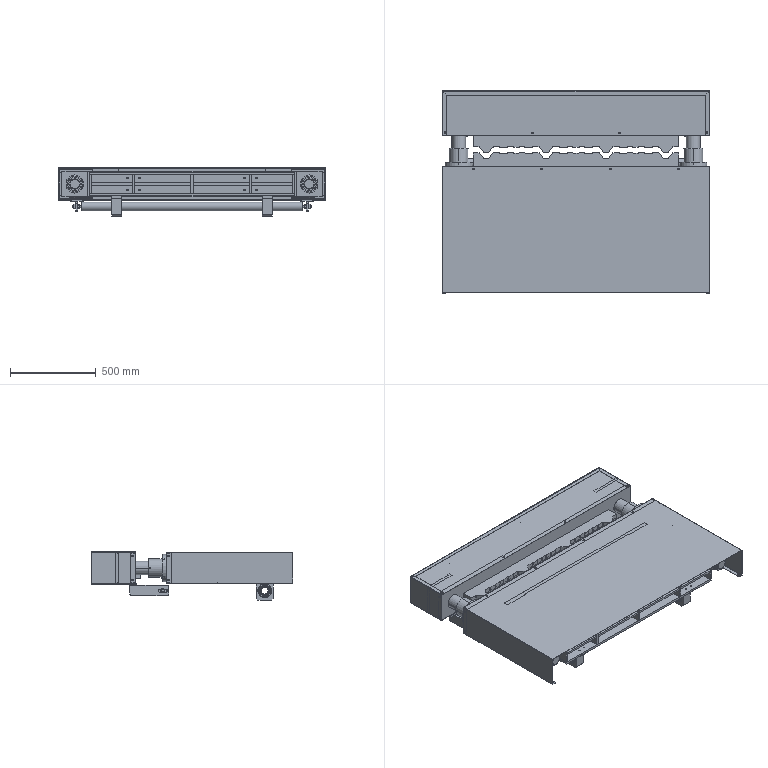Part | SolidWorks | 182 solids | 3799 faces | volume 91713160 mm3 | plane 1608 | cylinder 1221 | cone 590 | sphere 256 | torus 116 | spline 8 | commonest cylinder face diameters 7 x136 16 x116 58 x116 62 x116 10 x76 80 x76